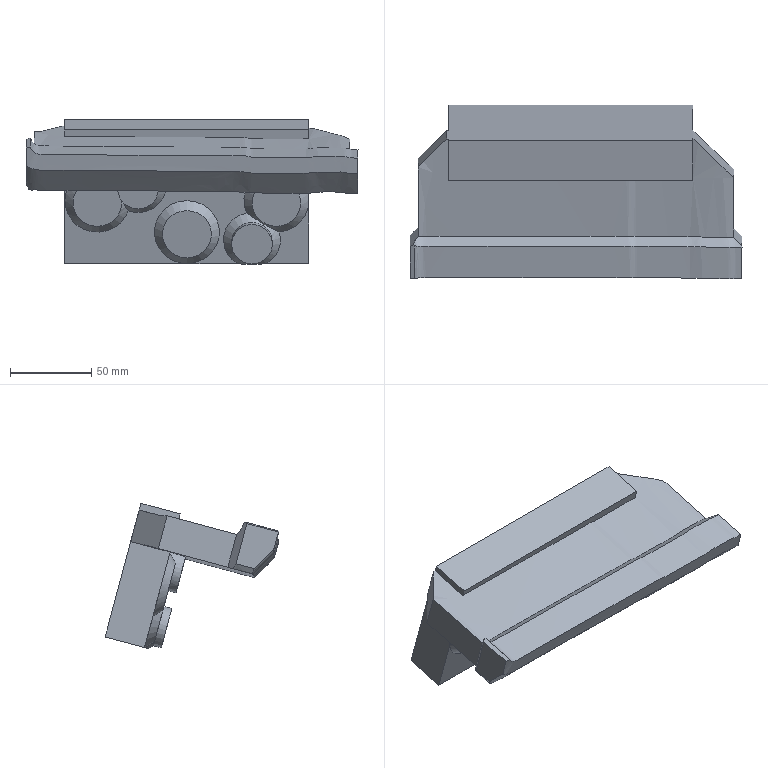Part | NX | features solid 2 | 1 solid | 40 faces | box 203.918 x 106.717 x 89.221 mm | volume 615293 mm3 | plane 26 | spline 7 | cone 5 | cylinder 2 | commonest cylinder face diameters 25 x2